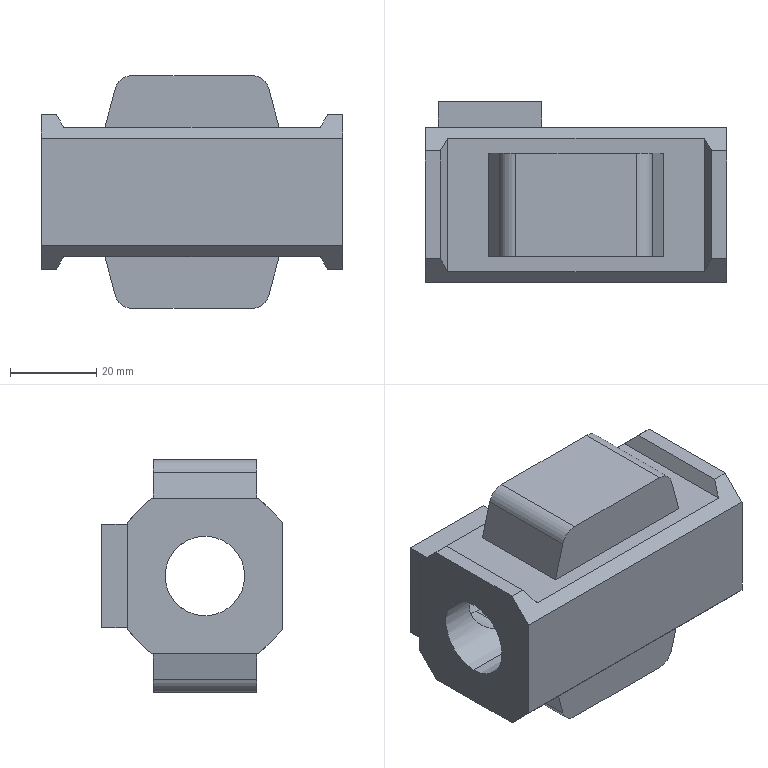Part | STEP file | AC40-04-KSTV-38JNR_AC3009A AKM Body | 1 solid | 46 faces | box 70 x 42 x 54 mm | volume 78893 mm3 | plane 34 | cylinder 8 | cone 4 | commonest cylinder face diameters 8 x4 14.5 x2 18.5 x2